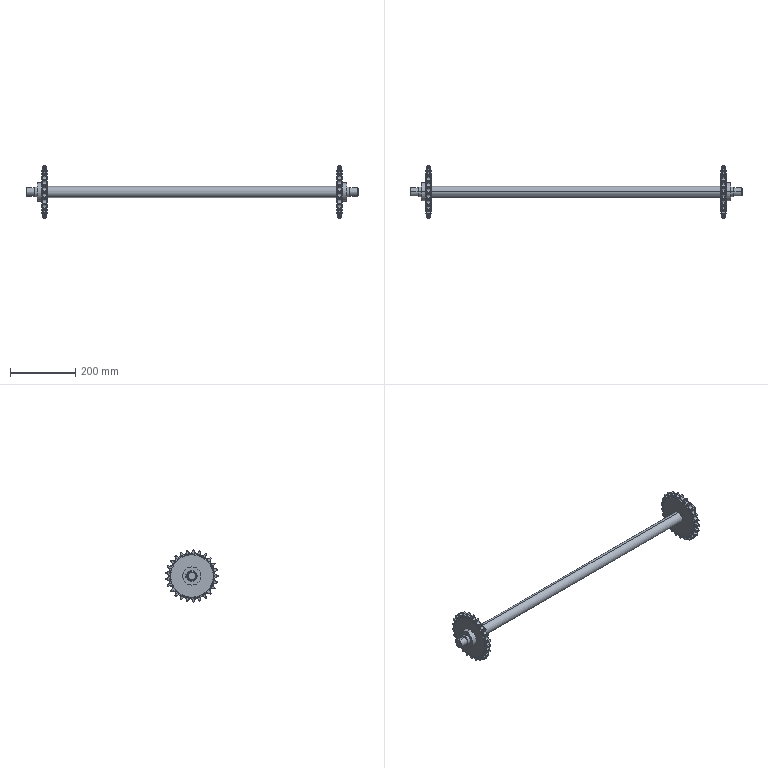Part | NX | features BREP 2 | 3 solids | 609 faces | box 1020 x 160.481 x 160.793 mm | volume 1435529 mm3 | cylinder 354 | plane 125 | torus 112 | cone 18 | commonest cylinder face diameters 17.202 x106 31.126 x104 12.07 x64 161 x50 30 x10 131 x8